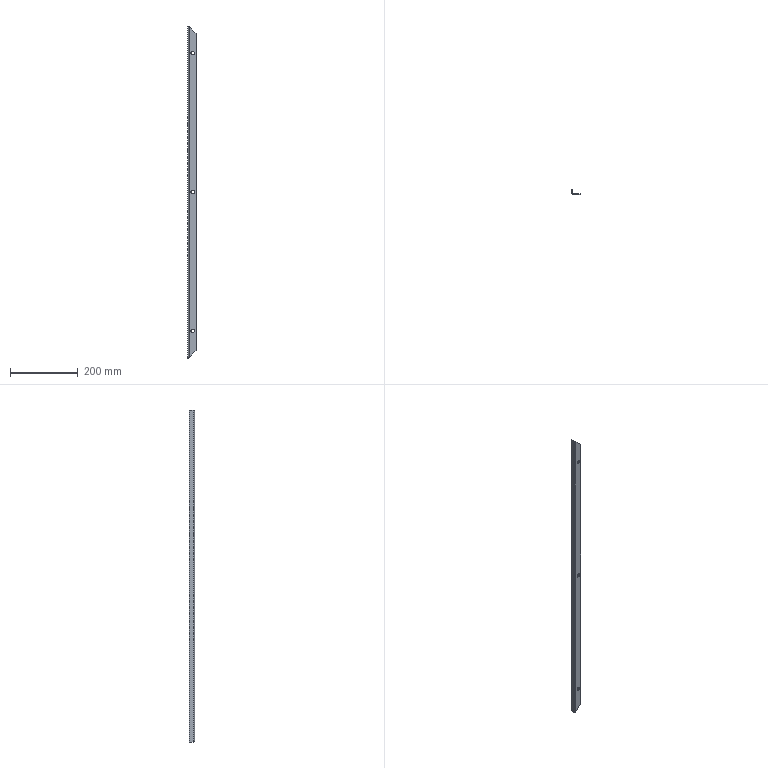Part | STEP file | 750038196 | 1 solid | 20 faces | box 24 x 15 x 981 mm | volume 68574 mm3 | plane 10 | cylinder 8 | spline 2 | commonest cylinder face diameters 10.5 x6 4 x1 8 x1
STEP:
#1=CARTESIAN_POINT('',(14.,2.,5.25));
#2=VERTEX_POINT('',#1);
#3=CARTESIAN_POINT('',(14.,2.,-5.25));
#4=VERTEX_POINT('',#3);
#5=CARTESIAN_POINT('',(14.,2.,0.));
#6=DIRECTION('',(0.,-1.,0.));
#7=DIRECTION('',(0.,0.,-1.));
#8=AXIS2_PLACEMENT_3D('',#5,#6,#7);
#9=CIRCLE('',#8,5.25);
#10=EDGE_CURVE('',#2,#4,#9,.T.);
#11=ORIENTED_EDGE('',*,*,#10,.F.);
#12=CARTESIAN_POINT('',(14.,0.,5.25));
#13=VERTEX_POINT('',#12);
#14=CARTESIAN_POINT('',(14.,981.408,5.25));
#15=DIRECTION('',(0.,-1.,0.));
#16=VECTOR('',#15,1000.);
#17=LINE('',#14,#16);
#18=EDGE_CURVE('',#2,#13,#17,.T.);
#19=ORIENTED_EDGE('',*,*,#18,.T.);
#20=CARTESIAN_POINT('',(14.,0.,-5.25));
#21=VERTEX_POINT('',#20);
#22=CARTESIAN_POINT('',(14.,0.,0.));
#23=DIRECTION('',(0.,1.,0.));
#24=DIRECTION('',(0.,0.,-1.));
#25=AXIS2_PLACEMENT_3D('',#22,#23,#24);
#26=CIRCLE('',#25,5.25);
#27=EDGE_CURVE('',#21,#13,#26,.T.);
#28=ORIENTED_EDGE('',*,*,#27,.F.);
#29=CARTESIAN_POINT('',(14.,981.408,-5.25));
#30=DIRECTION('',(0.,-1.,0.));
#31=VECTOR('',#30,1000.);
#32=LINE('',#29,#31);
#33=EDGE_CURVE('',#4,#21,#32,.T.);
#34=ORIENTED_EDGE('',*,*,#33,.F.);
#35=EDGE_LOOP('',(#11,#19,#28,#34));
#36=FACE_OUTER_BOUND('',#35,.T.);
#37=CARTESIAN_POINT('',(14.,981.408,0.));
#38=DIRECTION('',(0.,-1.,0.));
#39=DIRECTION('',(0.,0.,-1.));
#40=AXIS2_PLACEMENT_3D('',#37,#38,#39);
#41=CYLINDRICAL_SURFACE('',#40,5.25);
#42=ADVANCED_FACE('',(#36),#41,.F.);
#43=CARTESIAN_POINT('',(14.,2.,-405.25));
#44=VERTEX_POINT('',#43);
#45=CARTESIAN_POINT('',(14.,2.,-415.75));
#46=VERTEX_POINT('',#45);
#47=CARTESIAN_POINT('',(14.,2.,-410.5));
#48=DIRECTION('',(0.,-1.,0.));
#49=DIRECTION('',(0.,0.,-1.));
#50=AXIS2_PLACEMENT_3D('',#47,#48,#49);
#51=CIRCLE('',#50,5.25);
#52=EDGE_CURVE('',#44,#46,#51,.T.);
#53=ORIENTED_EDGE('',*,*,#52,.F.);
#54=CARTESIAN_POINT('',(14.,0.,-405.25));
#55=VERTEX_POINT('',#54);
#56=CARTESIAN_POINT('',(14.,981.408,-405.25));
#57=DIRECTION('',(0.,-1.,0.));
#58=VECTOR('',#57,1000.);
#59=LINE('',#56,#58);
#60=EDGE_CURVE('',#44,#55,#59,.T.);
#61=ORIENTED_EDGE('',*,*,#60,.T.);
#62=CARTESIAN_POINT('',(14.,0.,-415.75));
#63=VERTEX_POINT('',#62);
#64=CARTESIAN_POINT('',(14.,0.,-410.5));
#65=DIRECTION('',(0.,1.,0.));
#66=DIRECTION('',(0.,0.,-1.));
#67=AXIS2_PLACEMENT_3D('',#64,#65,#66);
#68=CIRCLE('',#67,5.25);
#69=EDGE_CURVE('',#63,#55,#68,.T.);
#70=ORIENTED_EDGE('',*,*,#69,.F.);
#71=CARTESIAN_POINT('',(14.,981.408,-415.75));
#72=DIRECTION('',(0.,-1.,0.));
#73=VECTOR('',#72,1000.);
#74=LINE('',#71,#73);
#75=EDGE_CURVE('',#46,#63,#74,.T.);
#76=ORIENTED_EDGE('',*,*,#75,.F.);
#77=EDGE_LOOP('',(#53,#61,#70,#76));
#78=FACE_OUTER_BOUND('',#77,.T.);
#79=CARTESIAN_POINT('',(14.,981.408,-410.5));
#80=DIRECTION('',(0.,-1.,0.));
#81=DIRECTION('',(0.,0.,-1.));
#82=AXIS2_PLACEMENT_3D('',#79,#80,#81);
#83=CYLINDRICAL_SURFACE('',#82,5.25);
#84=ADVANCED_FACE('',(#78),#83,.F.);
#85=CARTESIAN_POINT('',(14.,2.,415.75));
#86=VERTEX_POINT('',#85);
#87=CARTESIAN_POINT('',(14.,2.,405.25));
#88=VERTEX_POINT('',#87);
#89=CARTESIAN_POINT('',(14.,2.,410.5));
#90=DIRECTION('',(0.,-1.,0.));
#91=DIRECTION('',(0.,0.,-1.));
#92=AXIS2_PLACEMENT_3D('',#89,#90,#91);
#93=CIRCLE('',#92,5.25);
#94=EDGE_CURVE('',#86,#88,#93,.T.);
#95=ORIENTED_EDGE('',*,*,#94,.F.);
#96=CARTESIAN_POINT('',(14.,0.,415.75));
#97=VERTEX_POINT('',#96);
#98=CARTESIAN_POINT('',(14.,981.408,415.75));
#99=DIRECTION('',(0.,-1.,0.));
#100=VECTOR('',#99,1000.);
#101=LINE('',#98,#100);
#102=EDGE_CURVE('',#86,#97,#101,.T.);
#103=ORIENTED_EDGE('',*,*,#102,.T.);
#104=CARTESIAN_POINT('',(14.,0.,405.25));
#105=VERTEX_POINT('',#104);
#106=CARTESIAN_POINT('',(14.,0.,410.5));
#107=DIRECTION('',(0.,1.,0.));
#108=DIRECTION('',(0.,0.,-1.));
#109=AXIS2_PLACEMENT_3D('',#106,#107,#108);
#110=CIRCLE('',#109,5.25);
#111=EDGE_CURVE('',#105,#97,#110,.T.);
#112=ORIENTED_EDGE('',*,*,#111,.F.);
#113=CARTESIAN_POINT('',(14.,981.408,405.25));
#114=DIRECTION('',(0.,-1.,0.));
#115=VECTOR('',#114,1000.);
#116=LINE('',#113,#115);
#117=EDGE_CURVE('',#88,#105,#116,.T.);
#118=ORIENTED_EDGE('',*,*,#117,.F.);
#119=EDGE_LOOP('',(#95,#103,#112,#118));
#120=FACE_OUTER_BOUND('',#119,.T.);
#121=CARTESIAN_POINT('',(14.,981.408,410.5));
#122=DIRECTION('',(0.,-1.,0.));
#123=DIRECTION('',(0.,0.,-1.));
#124=AXIS2_PLACEMENT_3D('',#121,#122,#123);
#125=CYLINDRICAL_SURFACE('',#124,5.25);
#126=ADVANCED_FACE('',(#120),#125,.F.);
#127=CARTESIAN_POINT('',(4.,0.,488.5));
#128=VERTEX_POINT('',#127);
#129=CARTESIAN_POINT('',(4.,0.,-488.5));
#130=VERTEX_POINT('',#129);
#131=CARTESIAN_POINT('',(4.,0.,490.5));
#132=DIRECTION('',(0.,0.,-1.));
#133=VECTOR('',#132,1000.);
#134=LINE('',#131,#133);
#135=EDGE_CURVE('',#128,#130,#134,.T.);
#136=ORIENTED_EDGE('',*,*,#135,.T.);
#137=CARTESIAN_POINT('',(24.,0.,-468.5));
#138=VERTEX_POINT('',#137);
#139=CARTESIAN_POINT('',(4.,0.,-488.5));
#140=DIRECTION('',(0.7071,0.,0.7071));
#141=VECTOR('',#140,1000.);
#142=LINE('',#139,#141);
#143=EDGE_CURVE('',#130,#138,#142,.T.);
#144=ORIENTED_EDGE('',*,*,#143,.T.);
#145=CARTESIAN_POINT('',(24.,0.,468.5));
#146=VERTEX_POINT('',#145);
#147=CARTESIAN_POINT('',(24.,0.,490.5));
#148=DIRECTION('',(0.,0.,1.));
#149=VECTOR('',#148,1000.);
#150=LINE('',#147,#149);
#151=EDGE_CURVE('',#138,#146,#150,.T.);
#152=ORIENTED_EDGE('',*,*,#151,.T.);
#153=CARTESIAN_POINT('',(24.,0.,468.5));
#154=DIRECTION('',(-0.7071,0.,0.7071));
#155=VECTOR('',#154,1000.);
#156=LINE('',#153,#155);
#157=EDGE_CURVE('',#146,#128,#156,.T.);
#158=ORIENTED_EDGE('',*,*,#157,.T.);
#159=EDGE_LOOP('',(#136,#144,#152,#158));
#160=FACE_OUTER_BOUND('',#159,.T.);
#161=ORIENTED_EDGE('',*,*,#27,.T.);
#162=CARTESIAN_POINT('',(14.,0.,0.));
#163=DIRECTION('',(0.,1.,0.));
#164=DIRECTION('',(0.,0.,-1.));
#165=AXIS2_PLACEMENT_3D('',#162,#163,#164);
#166=CIRCLE('',#165,5.25);
#167=EDGE_CURVE('',#13,#21,#166,.T.);
#168=ORIENTED_EDGE('',*,*,#167,.T.);
#169=EDGE_LOOP('',(#161,#168));
#170=FACE_BOUND('',#169,.T.);
#171=ORIENTED_EDGE('',*,*,#69,.T.);
#172=CARTESIAN_POINT('',(14.,0.,-410.5));
#173=DIRECTION('',(0.,1.,0.));
#174=DIRECTION('',(0.,0.,-1.));
#175=AXIS2_PLACEMENT_3D('',#172,#173,#174);
#176=CIRCLE('',#175,5.25);
#177=EDGE_CURVE('',#55,#63,#176,.T.);
#178=ORIENTED_EDGE('',*,*,#177,.T.);
#179=EDGE_LOOP('',(#171,#178));
#180=FACE_BOUND('',#179,.T.);
#181=ORIENTED_EDGE('',*,*,#111,.T.);
#182=CARTESIAN_POINT('',(14.,0.,410.5));
#183=DIRECTION('',(0.,1.,0.));
#184=DIRECTION('',(0.,0.,-1.));
#185=AXIS2_PLACEMENT_3D('',#182,#183,#184);
#186=CIRCLE('',#185,5.25);
#187=EDGE_CURVE('',#97,#105,#186,.T.);
#188=ORIENTED_EDGE('',*,*,#187,.T.);
#189=EDGE_LOOP('',(#181,#188));
#190=FACE_BOUND('',#189,.T.);
#191=CARTESIAN_POINT('',(24.,0.,490.5));
#192=DIRECTION('',(0.,-1.,0.));
#193=DIRECTION('',(0.,0.,-1.));
#194=AXIS2_PLACEMENT_3D('',#191,#192,#193);
#195=PLANE('',#194);
#196=ADVANCED_FACE('',(#160,#170,#180,#190),#195,.T.);
#197=CARTESIAN_POINT('',(4.,2.,-488.5));
#198=VERTEX_POINT('',#197);
#199=CARTESIAN_POINT('',(4.,0.,-488.5));
#200=DIRECTION('',(0.,1.,0.));
#201=VECTOR('',#200,1000.);
#202=LINE('',#199,#201);
#203=EDGE_CURVE('',#130,#198,#202,.T.);
#204=ORIENTED_EDGE('',*,*,#203,.T.);
#205=CARTESIAN_POINT('',(24.,2.,-468.5));
#206=VERTEX_POINT('',#205);
#207=CARTESIAN_POINT('',(503.5,2.,11.));
#208=DIRECTION('',(0.7071,0.,0.7071));
#209=VECTOR('',#208,1000.);
#210=LINE('',#207,#209);
#211=EDGE_CURVE('',#198,#206,#210,.T.);
#212=ORIENTED_EDGE('',*,*,#211,.T.);
#213=CARTESIAN_POINT('',(24.,0.,-468.5));
#214=DIRECTION('',(0.,-1.,0.));
#215=VECTOR('',#214,1000.);
#216=LINE('',#213,#215);
#217=EDGE_CURVE('',#206,#138,#216,.T.);
#218=ORIENTED_EDGE('',*,*,#217,.T.);
#219=ORIENTED_EDGE('',*,*,#143,.F.);
#220=EDGE_LOOP('',(#204,#212,#218,#219));
#221=FACE_OUTER_BOUND('',#220,.T.);
#222=CARTESIAN_POINT('',(503.5,0.,11.));
#223=DIRECTION('',(0.7071,0.,-0.7071));
#224=DIRECTION('',(-0.7071,0.,-0.7071));
#225=AXIS2_PLACEMENT_3D('',#222,#223,#224);
#226=PLANE('',#225);
#227=ADVANCED_FACE('',(#221),#226,.T.);
#228=CARTESIAN_POINT('',(0.,4.,490.5));
#229=VERTEX_POINT('',#228);
#230=CARTESIAN_POINT('',(0.,4.,-490.5));
#231=VERTEX_POINT('',#230);
#232=CARTESIAN_POINT('',(0.,4.,490.5));
#233=DIRECTION('',(0.,0.,-1.));
#234=VECTOR('',#233,1000.);
#235=LINE('',#232,#234);
#236=EDGE_CURVE('',#229,#231,#235,.T.);
#237=ORIENTED_EDGE('',*,*,#236,.T.);
#238=CARTESIAN_POINT('',(0.,4.,-490.5));
#239=CARTESIAN_POINT('',(0.,2.,-490.5));
#240=CARTESIAN_POINT('',(1.333,0.,-489.833));
#241=CARTESIAN_POINT('',(4.,0.,-488.5));
#242=(BOUNDED_CURVE()B_SPLINE_CURVE(3,(#238,#239,#240,#241),.UNSPECIFIED.,.F.,.F.)B_SPLINE_CURVE_WITH_KNOTS((4,4),(0.,0.006627),.UNSPECIFIED.)CURVE()GEOMETRIC_REPRESENTATION_ITEM()RATIONAL_B_SPLINE_CURVE((1.,0.6667,0.5,0.5))REPRESENTATION_ITEM(''));
#243=EDGE_CURVE('',#231,#130,#242,.T.);
#244=ORIENTED_EDGE('',*,*,#243,.T.);
#245=ORIENTED_EDGE('',*,*,#135,.F.);
#246=CARTESIAN_POINT('',(4.,0.,488.5));
#247=CARTESIAN_POINT('',(1.333,0.,489.833));
#248=CARTESIAN_POINT('',(0.,2.,490.5));
#249=CARTESIAN_POINT('',(0.,4.,490.5));
#250=(BOUNDED_CURVE()B_SPLINE_CURVE(3,(#246,#247,#248,#249),.UNSPECIFIED.,.F.,.F.)B_SPLINE_CURVE_WITH_KNOTS((4,4),(0.,0.006641),.UNSPECIFIED.)CURVE()GEOMETRIC_REPRESENTATION_ITEM()RATIONAL_B_SPLINE_CURVE((0.5,0.5,0.6667,1.))REPRESENTATION_ITEM(''));
#251=EDGE_CURVE('',#128,#229,#250,.T.);
#252=ORIENTED_EDGE('',*,*,#251,.T.);
#253=EDGE_LOOP('',(#237,#244,#245,#252));
#254=FACE_OUTER_BOUND('',#253,.T.);
#255=CARTESIAN_POINT('',(4.,4.,490.5));
#256=DIRECTION('',(0.,0.,-1.));
#257=DIRECTION('',(-1.,0.,0.));
#258=AXIS2_PLACEMENT_3D('',#255,#256,#257);
#259=CYLINDRICAL_SURFACE('',#258,4.);
#260=ADVANCED_FACE('',(#254),#259,.T.);
#261=CARTESIAN_POINT('',(24.,2.,468.5));
#262=VERTEX_POINT('',#261);
#263=CARTESIAN_POINT('',(24.,0.,468.5));
#264=DIRECTION('',(0.,1.,0.));
#265=VECTOR('',#264,1000.);
#266=LINE('',#263,#265);
#267=EDGE_CURVE('',#146,#262,#266,.T.);
#268=ORIENTED_EDGE('',*,*,#267,.T.);
#269=CARTESIAN_POINT('',(4.,2.,488.5));
#270=VERTEX_POINT('',#269);
#271=CARTESIAN_POINT('',(13.,2.,479.5));
#272=DIRECTION('',(-0.7071,0.,0.7071));
#273=VECTOR('',#272,1000.);
#274=LINE('',#271,#273);
#275=EDGE_CURVE('',#262,#270,#274,.T.);
#276=ORIENTED_EDGE('',*,*,#275,.T.);
#277=CARTESIAN_POINT('',(4.,0.,488.5));
#278=DIRECTION('',(0.,-1.,0.));
#279=VECTOR('',#278,1000.);
#280=LINE('',#277,#279);
#281=EDGE_CURVE('',#270,#128,#280,.T.);
#282=ORIENTED_EDGE('',*,*,#281,.T.);
#283=ORIENTED_EDGE('',*,*,#157,.F.);
#284=EDGE_LOOP('',(#268,#276,#282,#283));
#285=FACE_OUTER_BOUND('',#284,.T.);
#286=CARTESIAN_POINT('',(13.,0.,479.5));
#287=DIRECTION('',(0.7071,0.,0.7071));
#288=DIRECTION('',(0.7071,0.,-0.7071));
#289=AXIS2_PLACEMENT_3D('',#286,#287,#288);
#290=PLANE('',#289);
#291=ADVANCED_FACE('',(#285),#290,.T.);
#292=ORIENTED_EDGE('',*,*,#267,.F.);
#293=ORIENTED_EDGE('',*,*,#151,.F.);
#294=ORIENTED_EDGE('',*,*,#217,.F.);
#295=CARTESIAN_POINT('',(24.,2.,490.5));
#296=DIRECTION('',(0.,0.,-1.));
#297=VECTOR('',#296,1000.);
#298=LINE('',#295,#297);
#299=EDGE_CURVE('',#262,#206,#298,.T.);
#300=ORIENTED_EDGE('',*,*,#299,.F.);
#301=EDGE_LOOP('',(#292,#293,#294,#300));
#302=FACE_OUTER_BOUND('',#301,.T.);
#303=CARTESIAN_POINT('',(24.,0.,490.5));
#304=DIRECTION('',(-1.,0.,0.));
#305=DIRECTION('',(0.,0.,1.));
#306=AXIS2_PLACEMENT_3D('',#303,#304,#305);
#307=PLANE('',#306);
#308=ADVANCED_FACE('',(#302),#307,.F.);
#309=ORIENTED_EDGE('',*,*,#18,.F.);
#310=CARTESIAN_POINT('',(14.,2.,0.));
#311=DIRECTION('',(0.,-1.,0.));
#312=DIRECTION('',(0.,0.,-1.));
#313=AXIS2_PLACEMENT_3D('',#310,#311,#312);
#314=CIRCLE('',#313,5.25);
#315=EDGE_CURVE('',#4,#2,#314,.T.);
#316=ORIENTED_EDGE('',*,*,#315,.F.);
#317=ORIENTED_EDGE('',*,*,#33,.T.);
#318=ORIENTED_EDGE('',*,*,#167,.F.);
#319=EDGE_LOOP('',(#309,#316,#317,#318));
#320=FACE_OUTER_BOUND('',#319,.T.);
#321=CARTESIAN_POINT('',(14.,981.408,0.));
#322=DIRECTION('',(0.,-1.,0.));
#323=DIRECTION('',(0.,0.,-1.));
#324=AXIS2_PLACEMENT_3D('',#321,#322,#323);
#325=CYLINDRICAL_SURFACE('',#324,5.25);
#326=ADVANCED_FACE('',(#320),#325,.F.);
#327=ORIENTED_EDGE('',*,*,#60,.F.);
#328=CARTESIAN_POINT('',(14.,2.,-410.5));
#329=DIRECTION('',(0.,-1.,0.));
#330=DIRECTION('',(0.,0.,-1.));
#331=AXIS2_PLACEMENT_3D('',#328,#329,#330);
#332=CIRCLE('',#331,5.25);
#333=EDGE_CURVE('',#46,#44,#332,.T.);
#334=ORIENTED_EDGE('',*,*,#333,.F.);
#335=ORIENTED_EDGE('',*,*,#75,.T.);
#336=ORIENTED_EDGE('',*,*,#177,.F.);
#337=EDGE_LOOP('',(#327,#334,#335,#336));
#338=FACE_OUTER_BOUND('',#337,.T.);
#339=CARTESIAN_POINT('',(14.,981.408,-410.5));
#340=DIRECTION('',(0.,-1.,0.));
#341=DIRECTION('',(0.,0.,-1.));
#342=AXIS2_PLACEMENT_3D('',#339,#340,#341);
#343=CYLINDRICAL_SURFACE('',#342,5.25);
#344=ADVANCED_FACE('',(#338),#343,.F.);
#345=ORIENTED_EDGE('',*,*,#102,.F.);
#346=CARTESIAN_POINT('',(14.,2.,410.5));
#347=DIRECTION('',(0.,-1.,0.));
#348=DIRECTION('',(0.,0.,-1.));
#349=AXIS2_PLACEMENT_3D('',#346,#347,#348);
#350=CIRCLE('',#349,5.25);
#351=EDGE_CURVE('',#88,#86,#350,.T.);
#352=ORIENTED_EDGE('',*,*,#351,.F.);
#353=ORIENTED_EDGE('',*,*,#117,.T.);
#354=ORIENTED_EDGE('',*,*,#187,.F.);
#355=EDGE_LOOP('',(#345,#352,#353,#354));
#356=FACE_OUTER_BOUND('',#355,.T.);
#357=CARTESIAN_POINT('',(14.,981.408,410.5));
#358=DIRECTION('',(0.,-1.,0.));
#359=DIRECTION('',(0.,0.,-1.));
#360=AXIS2_PLACEMENT_3D('',#357,#358,#359);
#361=CYLINDRICAL_SURFACE('',#360,5.25);
#362=ADVANCED_FACE('',(#356),#361,.F.);
#363=ORIENTED_EDGE('',*,*,#299,.T.);
#364=ORIENTED_EDGE('',*,*,#211,.F.);
#365=CARTESIAN_POINT('',(4.,2.,490.5));
#366=DIRECTION('',(0.,0.,-1.));
#367=VECTOR('',#366,1000.);
#368=LINE('',#365,#367);
#369=EDGE_CURVE('',#270,#198,#368,.T.);
#370=ORIENTED_EDGE('',*,*,#369,.F.);
#371=ORIENTED_EDGE('',*,*,#275,.F.);
#372=EDGE_LOOP('',(#363,#364,#370,#371));
#373=FACE_OUTER_BOUND('',#372,.T.);
#374=ORIENTED_EDGE('',*,*,#315,.T.);
#375=ORIENTED_EDGE('',*,*,#10,.T.);
#376=EDGE_LOOP('',(#374,#375));
#377=FACE_BOUND('',#376,.T.);
#378=ORIENTED_EDGE('',*,*,#333,.T.);
#379=ORIENTED_EDGE('',*,*,#52,.T.);
#380=EDGE_LOOP('',(#378,#379));
#381=FACE_BOUND('',#380,.T.);
#382=ORIENTED_EDGE('',*,*,#351,.T.);
#383=ORIENTED_EDGE('',*,*,#94,.T.);
#384=EDGE_LOOP('',(#382,#383));
#385=FACE_BOUND('',#384,.T.);
#386=CARTESIAN_POINT('',(24.,2.,490.5));
#387=DIRECTION('',(0.,-1.,0.));
#388=DIRECTION('',(0.,0.,-1.));
#389=AXIS2_PLACEMENT_3D('',#386,#387,#388);
#390=PLANE('',#389);
#391=ADVANCED_FACE('',(#373,#377,#381,#385),#390,.F.);
#392=CARTESIAN_POINT('',(2.,4.,-490.5));
#393=VERTEX_POINT('',#392);
#394=CARTESIAN_POINT('',(1.,4.,-490.5));
#395=DIRECTION('',(-1.,0.,0.));
#396=VECTOR('',#395,1000.);
#397=LINE('',#394,#396);
#398=EDGE_CURVE('',#393,#231,#397,.T.);
#399=ORIENTED_EDGE('',*,*,#398,.F.);
#400=CARTESIAN_POINT('',(4.,2.,-488.5));
#401=CARTESIAN_POINT('',(2.667,2.,-489.833));
#402=CARTESIAN_POINT('',(2.,3.,-490.5));
#403=CARTESIAN_POINT('',(2.,4.,-490.5));
#404=(BOUNDED_CURVE()B_SPLINE_CURVE(3,(#400,#401,#402,#403),.UNSPECIFIED.,.F.,.F.)B_SPLINE_CURVE_WITH_KNOTS((4,4),(0.,0.003785),.UNSPECIFIED.)CURVE()GEOMETRIC_REPRESENTATION_ITEM()RATIONAL_B_SPLINE_CURVE((0.5,0.5,0.6667,1.))REPRESENTATION_ITEM(''));
#405=EDGE_CURVE('',#198,#393,#404,.T.);
#406=ORIENTED_EDGE('',*,*,#405,.F.);
#407=ORIENTED_EDGE('',*,*,#203,.F.);
#408=ORIENTED_EDGE('',*,*,#243,.F.);
#409=EDGE_LOOP('',(#399,#406,#407,#408));
#410=FACE_OUTER_BOUND('',#409,.T.);
#411=CARTESIAN_POINT('',(0.,4.,-490.5));
#412=CARTESIAN_POINT('',(0.6667,4.,-490.5));
#413=CARTESIAN_POINT('',(1.333,4.,-490.5));
#414=CARTESIAN_POINT('',(2.,4.,-490.5));
#415=CARTESIAN_POINT('',(0.,-4.,-490.5));
#416=CARTESIAN_POINT('',(0.6667,-2.667,-490.5));
#417=CARTESIAN_POINT('',(1.333,-1.333,-490.5));
#418=CARTESIAN_POINT('',(2.,0.,-490.5));
#419=CARTESIAN_POINT('',(8.,-4.,-486.5));
#420=CARTESIAN_POINT('',(7.333,-2.667,-486.5));
#421=CARTESIAN_POINT('',(6.667,-1.333,-486.5));
#422=CARTESIAN_POINT('',(6.,0.,-486.5));
#423=CARTESIAN_POINT('',(8.,4.,-486.5));
#424=CARTESIAN_POINT('',(7.333,4.,-486.5));
#425=CARTESIAN_POINT('',(6.667,4.,-486.5));
#426=CARTESIAN_POINT('',(6.,4.,-486.5));
#427=CARTESIAN_POINT('',(8.,12.,-486.5));
#428=CARTESIAN_POINT('',(7.333,10.667,-486.5));
#429=CARTESIAN_POINT('',(6.667,9.333,-486.5));
#430=CARTESIAN_POINT('',(6.,8.,-486.5));
#431=CARTESIAN_POINT('',(0.,12.,-490.5));
#432=CARTESIAN_POINT('',(0.6667,10.667,-490.5));
#433=CARTESIAN_POINT('',(1.333,9.333,-490.5));
#434=CARTESIAN_POINT('',(2.,8.,-490.5));
#435=CARTESIAN_POINT('',(0.,4.,-490.5));
#436=CARTESIAN_POINT('',(0.6667,4.,-490.5));
#437=CARTESIAN_POINT('',(1.333,4.,-490.5));
#438=CARTESIAN_POINT('',(2.,4.,-490.5));
#439=(BOUNDED_SURFACE()B_SPLINE_SURFACE(3,3,((#411,#412,#413,#414),(#415,#416,#417,#418),(#419,#420,#421,#422),(#423,#424,#425,#426),(#427,#428,#429,#430),(#431,#432,#433,#434),(#435,#436,#437,#438)),.UNSPECIFIED.,.T.,.F.,.F.)B_SPLINE_SURFACE_WITH_KNOTS((4,3,4),(4,4),(0.,0.5,1.),(0.,1.),.UNSPECIFIED.)GEOMETRIC_REPRESENTATION_ITEM()RATIONAL_B_SPLINE_SURFACE(((1.,1.,1.,1.),(0.3333,0.3333,0.3333,0.3333),(0.3333,0.3333,0.3333,0.3333),(1.,1.,1.,1.),(0.3333,0.3333,0.3333,0.3333),(0.3333,0.3333,0.3333,0.3333),(1.,1.,1.,1.)))REPRESENTATION_ITEM('')SURFACE());
#440=ADVANCED_FACE('',(#410),#439,.F.);
#441=CARTESIAN_POINT('',(0.,15.,490.5));
#442=VERTEX_POINT('',#441);
#443=CARTESIAN_POINT('',(0.,0.,490.5));
#444=DIRECTION('',(0.,1.,0.));
#445=VECTOR('',#444,1000.);
#446=LINE('',#443,#445);
#447=EDGE_CURVE('',#229,#442,#446,.T.);
#448=ORIENTED_EDGE('',*,*,#447,.T.);
#449=CARTESIAN_POINT('',(0.,15.,-490.5));
#450=VERTEX_POINT('',#449);
#451=CARTESIAN_POINT('',(0.,15.,490.5));
#452=DIRECTION('',(0.,0.,-1.));
#453=VECTOR('',#452,1000.);
#454=LINE('',#451,#453);
#455=EDGE_CURVE('',#442,#450,#454,.T.);
#456=ORIENTED_EDGE('',*,*,#455,.T.);
#457=CARTESIAN_POINT('',(0.,0.,-490.5));
#458=DIRECTION('',(0.,-1.,0.));
#459=VECTOR('',#458,1000.);
#460=LINE('',#457,#459);
#461=EDGE_CURVE('',#450,#231,#460,.T.);
#462=ORIENTED_EDGE('',*,*,#461,.T.);
#463=ORIENTED_EDGE('',*,*,#236,.F.);
#464=EDGE_LOOP('',(#448,#456,#462,#463));
#465=FACE_OUTER_BOUND('',#464,.T.);
#466=CARTESIAN_POINT('',(0.,0.,490.5));
#467=DIRECTION('',(-1.,0.,0.));
#468=DIRECTION('',(0.,-1.,0.));
#469=AXIS2_PLACEMENT_3D('',#466,#467,#468);
#470=PLANE('',#469);
#471=ADVANCED_FACE('',(#465),#470,.T.);
#472=CARTESIAN_POINT('',(2.,4.,490.5));
#473=VERTEX_POINT('',#472);
#474=CARTESIAN_POINT('',(2.,4.,490.5));
#475=CARTESIAN_POINT('',(2.,3.,490.5));
#476=CARTESIAN_POINT('',(2.667,2.,489.833));
#477=CARTESIAN_POINT('',(4.,2.,488.5));
#478=(BOUNDED_CURVE()B_SPLINE_CURVE(3,(#474,#475,#476,#477),.UNSPECIFIED.,.F.,.F.)B_SPLINE_CURVE_WITH_KNOTS((4,4),(0.,0.003806),.UNSPECIFIED.)CURVE()GEOMETRIC_REPRESENTATION_ITEM()RATIONAL_B_SPLINE_CURVE((1.,0.6667,0.5,0.5))REPRESENTATION_ITEM(''));
#479=EDGE_CURVE('',#473,#270,#478,.T.);
#480=ORIENTED_EDGE('',*,*,#479,.F.);
#481=CARTESIAN_POINT('',(1.,4.,490.5));
#482=DIRECTION('',(1.,0.,0.));
#483=VECTOR('',#482,1000.);
#484=LINE('',#481,#483);
#485=EDGE_CURVE('',#229,#473,#484,.T.);
#486=ORIENTED_EDGE('',*,*,#485,.F.);
#487=ORIENTED_EDGE('',*,*,#251,.F.);
#488=ORIENTED_EDGE('',*,*,#281,.F.);
#489=EDGE_LOOP('',(#480,#486,#487,#488));
#490=FACE_OUTER_BOUND('',#489,.T.);
#491=CARTESIAN_POINT('',(8.,4.,486.5));
#492=CARTESIAN_POINT('',(7.333,4.,486.5));
#493=CARTESIAN_POINT('',(6.667,4.,486.5));
#494=CARTESIAN_POINT('',(6.,4.,486.5));
#495=CARTESIAN_POINT('',(8.,-4.,486.5));
#496=CARTESIAN_POINT('',(7.333,-2.667,486.5));
#497=CARTESIAN_POINT('',(6.667,-1.333,486.5));
#498=CARTESIAN_POINT('',(6.,0.,486.5));
#499=CARTESIAN_POINT('',(0.,-4.,490.5));
#500=CARTESIAN_POINT('',(0.6667,-2.667,490.5));
#501=CARTESIAN_POINT('',(1.333,-1.333,490.5));
#502=CARTESIAN_POINT('',(2.,0.,490.5));
#503=CARTESIAN_POINT('',(0.,4.,490.5));
#504=CARTESIAN_POINT('',(0.6667,4.,490.5));
#505=CARTESIAN_POINT('',(1.333,4.,490.5));
#506=CARTESIAN_POINT('',(2.,4.,490.5));
#507=CARTESIAN_POINT('',(0.,12.,490.5));
#508=CARTESIAN_POINT('',(0.6667,10.667,490.5));
#509=CARTESIAN_POINT('',(1.333,9.333,490.5));
#510=CARTESIAN_POINT('',(2.,8.,490.5));
#511=CARTESIAN_POINT('',(8.,12.,486.5));
#512=CARTESIAN_POINT('',(7.333,10.667,486.5));
#513=CARTESIAN_POINT('',(6.667,9.333,486.5));
#514=CARTESIAN_POINT('',(6.,8.,486.5));
#515=CARTESIAN_POINT('',(8.,4.,486.5));
#516=CARTESIAN_POINT('',(7.333,4.,486.5));
#517=CARTESIAN_POINT('',(6.667,4.,486.5));
#518=CARTESIAN_POINT('',(6.,4.,486.5));
#519=(BOUNDED_SURFACE()B_SPLINE_SURFACE(3,3,((#491,#492,#493,#494),(#495,#496,#497,#498),(#499,#500,#501,#502),(#503,#504,#505,#506),(#507,#508,#509,#510),(#511,#512,#513,#514),(#515,#516,#517,#518)),.UNSPECIFIED.,.T.,.F.,.F.)B_SPLINE_SURFACE_WITH_KNOTS((4,3,4),(4,4),(0.,0.5,1.),(0.,1.),.UNSPECIFIED.)GEOMETRIC_REPRESENTATION_ITEM()RATIONAL_B_SPLINE_SURFACE(((1.,1.,1.,1.),(0.3333,0.3333,0.3333,0.3333),(0.3333,0.3333,0.3333,0.3333),(1.,1.,1.,1.),(0.3333,0.3333,0.3333,0.3333),(0.3333,0.3333,0.3333,0.3333),(1.,1.,1.,1.)))REPRESENTATION_ITEM('')SURFACE());
#520=ADVANCED_FACE('',(#490),#519,.F.);
#521=ORIENTED_EDGE('',*,*,#369,.T.);
#522=ORIENTED_EDGE('',*,*,#405,.T.);
#523=CARTESIAN_POINT('',(2.,4.,490.5));
#524=DIRECTION('',(0.,0.,-1.));
#525=VECTOR('',#524,1000.);
#526=LINE('',#523,#525);
#527=EDGE_CURVE('',#473,#393,#526,.T.);
#528=ORIENTED_EDGE('',*,*,#527,.F.);
#529=ORIENTED_EDGE('',*,*,#479,.T.);
#530=EDGE_LOOP('',(#521,#522,#528,#529));
#531=FACE_OUTER_BOUND('',#530,.T.);
#532=CARTESIAN_POINT('',(4.,4.,490.5));
#533=DIRECTION('',(0.,0.,-1.));
#534=DIRECTION('',(-1.,0.,0.));
#535=AXIS2_PLACEMENT_3D('',#532,#533,#534);
#536=CYLINDRICAL_SURFACE('',#535,2.);
#537=ADVANCED_FACE('',(#531),#536,.F.);
#538=ORIENTED_EDGE('',*,*,#461,.F.);
#539=CARTESIAN_POINT('',(2.,15.,-490.5));
#540=VERTEX_POINT('',#539);
#541=CARTESIAN_POINT('',(24.,15.,-490.5));
#542=DIRECTION('',(-1.,0.,0.));
#543=VECTOR('',#542,1000.);
#544=LINE('',#541,#543);
#545=EDGE_CURVE('',#540,#450,#544,.T.);
#546=ORIENTED_EDGE('',*,*,#545,.F.);
#547=CARTESIAN_POINT('',(2.,0.,-490.5));
#548=DIRECTION('',(0.,1.,0.));
#549=VECTOR('',#548,1000.);
#550=LINE('',#547,#549);
#551=EDGE_CURVE('',#393,#540,#550,.T.);
#552=ORIENTED_EDGE('',*,*,#551,.F.);
#553=ORIENTED_EDGE('',*,*,#398,.T.);
#554=EDGE_LOOP('',(#538,#546,#552,#553));
#555=FACE_OUTER_BOUND('',#554,.T.);
#556=CARTESIAN_POINT('',(24.,0.,-490.5));
#557=DIRECTION('',(0.,0.,1.));
#558=DIRECTION('',(1.,0.,0.));
#559=AXIS2_PLACEMENT_3D('',#556,#557,#558);
#560=PLANE('',#559);
#561=ADVANCED_FACE('',(#555),#560,.F.);
#562=ORIENTED_EDGE('',*,*,#545,.T.);
#563=ORIENTED_EDGE('',*,*,#455,.F.);
#564=CARTESIAN_POINT('',(2.,15.,490.5));
#565=VERTEX_POINT('',#564);
#566=CARTESIAN_POINT('',(0.,15.,490.5));
#567=DIRECTION('',(1.,0.,0.));
#568=VECTOR('',#567,1000.);
#569=LINE('',#566,#568);
#570=EDGE_CURVE('',#442,#565,#569,.T.);
#571=ORIENTED_EDGE('',*,*,#570,.T.);
#572=CARTESIAN_POINT('',(2.,15.,490.5));
#573=DIRECTION('',(0.,0.,-1.));
#574=VECTOR('',#573,1000.);
#575=LINE('',#572,#574);
#576=EDGE_CURVE('',#565,#540,#575,.T.);
#577=ORIENTED_EDGE('',*,*,#576,.T.);
#578=EDGE_LOOP('',(#562,#563,#571,#577));
#579=FACE_OUTER_BOUND('',#578,.T.);
#580=CARTESIAN_POINT('',(0.,15.,490.5));
#581=DIRECTION('',(0.,1.,0.));
#582=DIRECTION('',(-1.,0.,0.));
#583=AXIS2_PLACEMENT_3D('',#580,#581,#582);
#584=PLANE('',#583);
#585=ADVANCED_FACE('',(#579),#584,.T.);
#586=CARTESIAN_POINT('',(2.,0.,490.5));
#587=DIRECTION('',(0.,1.,0.));
#588=VECTOR('',#587,1000.);
#589=LINE('',#586,#588);
#590=EDGE_CURVE('',#473,#565,#589,.T.);
#591=ORIENTED_EDGE('',*,*,#590,.T.);
#592=ORIENTED_EDGE('',*,*,#570,.F.);
#593=ORIENTED_EDGE('',*,*,#447,.F.);
#594=ORIENTED_EDGE('',*,*,#485,.T.);
#595=EDGE_LOOP('',(#591,#592,#593,#594));
#596=FACE_OUTER_BOUND('',#595,.T.);
#597=CARTESIAN_POINT('',(0.,0.,490.5));
#598=DIRECTION('',(0.,0.,1.));
#599=DIRECTION('',(1.,0.,0.));
#600=AXIS2_PLACEMENT_3D('',#597,#598,#599);
#601=PLANE('',#600);
#602=ADVANCED_FACE('',(#596),#601,.T.);
#603=ORIENTED_EDGE('',*,*,#576,.F.);
#604=ORIENTED_EDGE('',*,*,#590,.F.);
#605=ORIENTED_EDGE('',*,*,#527,.T.);
#606=ORIENTED_EDGE('',*,*,#551,.T.);
#607=EDGE_LOOP('',(#603,#604,#605,#606));
#608=FACE_OUTER_BOUND('',#607,.T.);
#609=CARTESIAN_POINT('',(2.,0.,490.5));
#610=DIRECTION('',(-1.,0.,0.));
#611=DIRECTION('',(0.,-1.,0.));
#612=AXIS2_PLACEMENT_3D('',#609,#610,#611);
#613=PLANE('',#612);
#614=ADVANCED_FACE('',(#608),#613,.F.);
#615=CLOSED_SHELL('',(#42,#84,#126,#196,#227,#260,#291,#308,#326,#344,#362,#391,#440,#471,#520,#537,#561,#585,#602,#614));
#616=MANIFOLD_SOLID_BREP('',#615);
#617=CARTESIAN_POINT('',(0.,0.,0.));
#618=DIRECTION('',(0.,0.,1.));
#619=DIRECTION('',(1.,0.,0.));
#620=AXIS2_PLACEMENT_3D('',#617,#618,#619);
#621=(LENGTH_UNIT()NAMED_UNIT(*)SI_UNIT(.MILLI.,.METRE.));
#622=UNCERTAINTY_MEASURE_WITH_UNIT(LENGTH_MEASURE(0.00001),#621,'','');
#623=(NAMED_UNIT(*)PLANE_ANGLE_UNIT()SI_UNIT($,.RADIAN.));
#624=(NAMED_UNIT(*)SI_UNIT($,.STERADIAN.)SOLID_ANGLE_UNIT());
#625=(GEOMETRIC_REPRESENTATION_CONTEXT(3)GLOBAL_UNCERTAINTY_ASSIGNED_CONTEXT((#622))GLOBAL_UNIT_ASSIGNED_CONTEXT((#621,#623,#624))REPRESENTATION_CONTEXT('',''));
#626=ADVANCED_BREP_SHAPE_REPRESENTATION('',(#616,#620),#625);